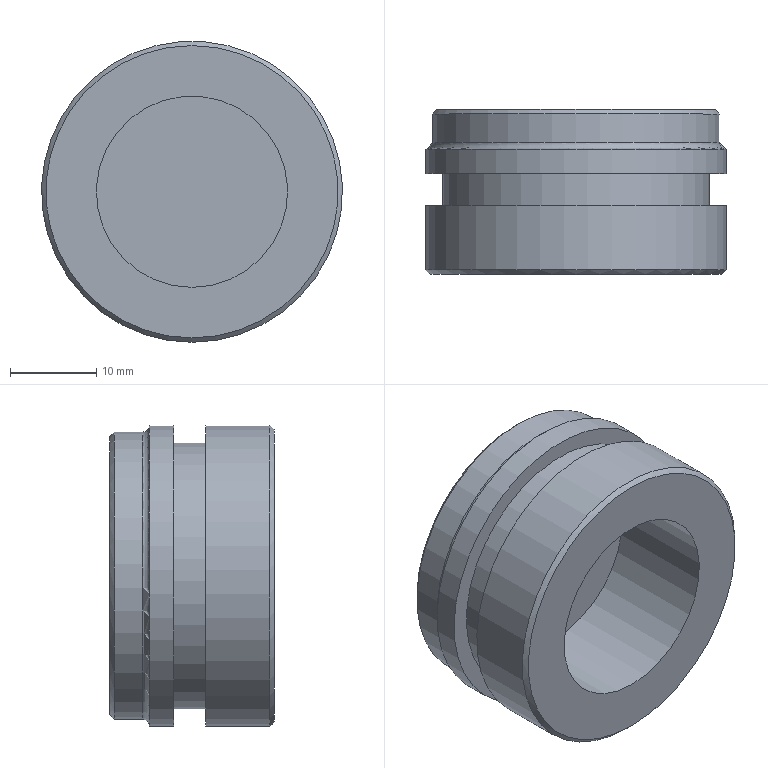Part | NX | features MG0330 trunion parts 24(stanchion group) 2 | 1 solid | 13 faces | box 34.849 x 19.05 x 34.849 mm | volume 12105 mm3 | cylinder 5 | plane 5 | cone 2 | torus 1 | commonest cylinder face diameters 34.849 x2 22.149 x1 30.836 x1 33.261 x1
STEP:
#1=CARTESIAN_POINT('',(0.,267.208,-17.424));
#2=VERTEX_POINT('',#1);
#3=CARTESIAN_POINT('',(0.,267.208,0.));
#4=DIRECTION('',(0.,-1.,0.));
#5=DIRECTION('',(0.,0.,-1.));
#6=AXIS2_PLACEMENT_3D('',#3,#4,#5);
#7=CIRCLE('',#6,17.424);
#8=EDGE_CURVE('',#2,#2,#7,.F.);
#9=ORIENTED_EDGE('',*,*,#8,.T.);
#10=EDGE_LOOP('',(#9));
#11=FACE_BOUND('',#10,.T.);
#12=CARTESIAN_POINT('',(0.,274.65,-17.424));
#13=VERTEX_POINT('',#12);
#14=CARTESIAN_POINT('',(0.,274.65,0.));
#15=DIRECTION('',(0.,-1.,0.));
#16=DIRECTION('',(0.,0.,-1.));
#17=AXIS2_PLACEMENT_3D('',#14,#15,#16);
#18=CIRCLE('',#17,17.424);
#19=EDGE_CURVE('',#13,#13,#18,.T.);
#20=ORIENTED_EDGE('',*,*,#19,.T.);
#21=EDGE_LOOP('',(#20));
#22=FACE_BOUND('',#21,.T.);
#23=CARTESIAN_POINT('',(0.,276.225,0.));
#24=DIRECTION('',(0.,-1.,0.));
#25=DIRECTION('',(0.,0.,-1.));
#26=AXIS2_PLACEMENT_3D('',#23,#24,#25);
#27=CYLINDRICAL_SURFACE('',#26,17.424);
#28=ADVANCED_FACE('',(#11,#22),#27,.T.);
#29=CARTESIAN_POINT('',(0.,274.65,-15.418));
#30=VERTEX_POINT('',#29);
#31=CARTESIAN_POINT('',(0.,274.65,0.));
#32=DIRECTION('',(0.,-1.,0.));
#33=DIRECTION('',(0.,0.,-1.));
#34=AXIS2_PLACEMENT_3D('',#31,#32,#33);
#35=CIRCLE('',#34,15.418);
#36=EDGE_CURVE('',#30,#30,#35,.T.);
#37=ORIENTED_EDGE('',*,*,#36,.T.);
#38=EDGE_LOOP('',(#37));
#39=FACE_BOUND('',#38,.T.);
#40=ORIENTED_EDGE('',*,*,#19,.F.);
#41=EDGE_LOOP('',(#40));
#42=FACE_BOUND('',#41,.T.);
#43=CARTESIAN_POINT('',(17.424,274.65,0.));
#44=DIRECTION('',(0.,1.,0.));
#45=DIRECTION('',(0.,0.,1.));
#46=AXIS2_PLACEMENT_3D('',#43,#44,#45);
#47=PLANE('',#46);
#48=ADVANCED_FACE('',(#39,#42),#47,.T.);
#49=CARTESIAN_POINT('',(0.,278.359,-15.418));
#50=VERTEX_POINT('',#49);
#51=CARTESIAN_POINT('',(0.,278.359,0.));
#52=DIRECTION('',(0.,-1.,0.));
#53=DIRECTION('',(0.,0.,-1.));
#54=AXIS2_PLACEMENT_3D('',#51,#52,#53);
#55=CIRCLE('',#54,15.418);
#56=EDGE_CURVE('',#50,#50,#55,.T.);
#57=ORIENTED_EDGE('',*,*,#56,.T.);
#58=EDGE_LOOP('',(#57));
#59=FACE_BOUND('',#58,.T.);
#60=ORIENTED_EDGE('',*,*,#36,.F.);
#61=EDGE_LOOP('',(#60));
#62=FACE_BOUND('',#61,.T.);
#63=CARTESIAN_POINT('',(0.,276.225,0.));
#64=DIRECTION('',(0.,-1.,0.));
#65=DIRECTION('',(0.,0.,-1.));
#66=AXIS2_PLACEMENT_3D('',#63,#64,#65);
#67=CYLINDRICAL_SURFACE('',#66,15.418);
#68=ADVANCED_FACE('',(#59,#62),#67,.T.);
#69=CARTESIAN_POINT('',(0.,278.359,-17.424));
#70=VERTEX_POINT('',#69);
#71=CARTESIAN_POINT('',(0.,278.359,0.));
#72=DIRECTION('',(0.,-1.,0.));
#73=DIRECTION('',(0.,0.,-1.));
#74=AXIS2_PLACEMENT_3D('',#71,#72,#73);
#75=CIRCLE('',#74,17.424);
#76=EDGE_CURVE('',#70,#70,#75,.T.);
#77=ORIENTED_EDGE('',*,*,#76,.T.);
#78=EDGE_LOOP('',(#77));
#79=FACE_BOUND('',#78,.T.);
#80=ORIENTED_EDGE('',*,*,#56,.F.);
#81=EDGE_LOOP('',(#80));
#82=FACE_BOUND('',#81,.T.);
#83=CARTESIAN_POINT('',(17.424,278.359,0.));
#84=DIRECTION('',(0.,-1.,0.));
#85=DIRECTION('',(0.,0.,-1.));
#86=AXIS2_PLACEMENT_3D('',#83,#84,#85);
#87=PLANE('',#86);
#88=ADVANCED_FACE('',(#79,#82),#87,.T.);
#89=CARTESIAN_POINT('',(0.,281.146,-17.424));
#90=VERTEX_POINT('',#89);
#91=CARTESIAN_POINT('',(0.,281.146,0.));
#92=DIRECTION('',(0.,-1.,0.));
#93=DIRECTION('',(0.,0.,-1.));
#94=AXIS2_PLACEMENT_3D('',#91,#92,#93);
#95=CIRCLE('',#94,17.424);
#96=EDGE_CURVE('',#90,#90,#95,.T.);
#97=ORIENTED_EDGE('',*,*,#96,.T.);
#98=EDGE_LOOP('',(#97));
#99=FACE_BOUND('',#98,.T.);
#100=ORIENTED_EDGE('',*,*,#76,.F.);
#101=EDGE_LOOP('',(#100));
#102=FACE_BOUND('',#101,.T.);
#103=CARTESIAN_POINT('',(0.,276.225,0.));
#104=DIRECTION('',(0.,-1.,0.));
#105=DIRECTION('',(0.,0.,-1.));
#106=AXIS2_PLACEMENT_3D('',#103,#104,#105);
#107=CYLINDRICAL_SURFACE('',#106,17.424);
#108=ADVANCED_FACE('',(#99,#102),#107,.T.);
#109=CARTESIAN_POINT('',(0.,281.94,-16.631));
#110=VERTEX_POINT('',#109);
#111=CARTESIAN_POINT('',(0.,281.94,0.));
#112=DIRECTION('',(0.,-1.,0.));
#113=DIRECTION('',(0.,0.,-1.));
#114=AXIS2_PLACEMENT_3D('',#111,#112,#113);
#115=CIRCLE('',#114,16.631);
#116=EDGE_CURVE('',#110,#110,#115,.T.);
#117=ORIENTED_EDGE('',*,*,#116,.T.);
#118=EDGE_LOOP('',(#117));
#119=FACE_BOUND('',#118,.T.);
#120=ORIENTED_EDGE('',*,*,#96,.F.);
#121=EDGE_LOOP('',(#120));
#122=FACE_BOUND('',#121,.T.);
#123=CARTESIAN_POINT('',(0.,281.94,0.));
#124=DIRECTION('',(0.,-1.,0.));
#125=DIRECTION('',(0.,0.,-1.));
#126=AXIS2_PLACEMENT_3D('',#123,#124,#125);
#127=TOROIDAL_SURFACE('',#126,17.424,0.7937);
#128=ADVANCED_FACE('',(#119,#122),#127,.F.);
#129=CARTESIAN_POINT('',(0.,285.242,16.631));
#130=VERTEX_POINT('',#129);
#131=CARTESIAN_POINT('',(0.,285.242,0.));
#132=DIRECTION('',(0.,1.,0.));
#133=DIRECTION('',(0.,0.,1.));
#134=AXIS2_PLACEMENT_3D('',#131,#132,#133);
#135=CIRCLE('',#134,16.631);
#136=EDGE_CURVE('',#130,#130,#135,.F.);
#137=ORIENTED_EDGE('',*,*,#136,.T.);
#138=EDGE_LOOP('',(#137));
#139=FACE_BOUND('',#138,.T.);
#140=ORIENTED_EDGE('',*,*,#116,.F.);
#141=EDGE_LOOP('',(#140));
#142=FACE_BOUND('',#141,.T.);
#143=CARTESIAN_POINT('',(0.,276.225,0.));
#144=DIRECTION('',(0.,-1.,0.));
#145=DIRECTION('',(0.,0.,-1.));
#146=AXIS2_PLACEMENT_3D('',#143,#144,#145);
#147=CYLINDRICAL_SURFACE('',#146,16.631);
#148=ADVANCED_FACE('',(#139,#142),#147,.T.);
#149=CARTESIAN_POINT('',(0.,285.75,16.123));
#150=VERTEX_POINT('',#149);
#151=CARTESIAN_POINT('',(0.,285.75,0.));
#152=DIRECTION('',(0.,1.,0.));
#153=DIRECTION('',(0.,0.,1.));
#154=AXIS2_PLACEMENT_3D('',#151,#152,#153);
#155=CIRCLE('',#154,16.123);
#156=EDGE_CURVE('',#150,#150,#155,.T.);
#157=ORIENTED_EDGE('',*,*,#156,.T.);
#158=EDGE_LOOP('',(#157));
#159=FACE_BOUND('',#158,.T.);
#160=CARTESIAN_POINT('',(16.631,285.75,0.));
#161=DIRECTION('',(0.,1.,0.));
#162=DIRECTION('',(0.,0.,1.));
#163=AXIS2_PLACEMENT_3D('',#160,#161,#162);
#164=PLANE('',#163);
#165=ADVANCED_FACE('',(#159),#164,.T.);
#166=CARTESIAN_POINT('',(0.,279.4,-11.074));
#167=VERTEX_POINT('',#166);
#168=CARTESIAN_POINT('',(0.,279.4,0.));
#169=DIRECTION('',(0.,-1.,0.));
#170=DIRECTION('',(0.,0.,-1.));
#171=AXIS2_PLACEMENT_3D('',#168,#169,#170);
#172=CIRCLE('',#171,11.074);
#173=EDGE_CURVE('',#167,#167,#172,.T.);
#174=ORIENTED_EDGE('',*,*,#173,.T.);
#175=EDGE_LOOP('',(#174));
#176=FACE_BOUND('',#175,.T.);
#177=CARTESIAN_POINT('',(11.074,279.4,0.));
#178=DIRECTION('',(0.,-1.,0.));
#179=DIRECTION('',(0.,0.,-1.));
#180=AXIS2_PLACEMENT_3D('',#177,#178,#179);
#181=PLANE('',#180);
#182=ADVANCED_FACE('',(#176),#181,.T.);
#183=CARTESIAN_POINT('',(0.,266.7,-11.074));
#184=VERTEX_POINT('',#183);
#185=CARTESIAN_POINT('',(0.,266.7,0.));
#186=DIRECTION('',(0.,-1.,0.));
#187=DIRECTION('',(0.,0.,-1.));
#188=AXIS2_PLACEMENT_3D('',#185,#186,#187);
#189=CIRCLE('',#188,11.074);
#190=EDGE_CURVE('',#184,#184,#189,.T.);
#191=ORIENTED_EDGE('',*,*,#190,.T.);
#192=EDGE_LOOP('',(#191));
#193=FACE_BOUND('',#192,.T.);
#194=ORIENTED_EDGE('',*,*,#173,.F.);
#195=EDGE_LOOP('',(#194));
#196=FACE_BOUND('',#195,.T.);
#197=CARTESIAN_POINT('',(0.,276.225,0.));
#198=DIRECTION('',(0.,-1.,0.));
#199=DIRECTION('',(0.,0.,-1.));
#200=AXIS2_PLACEMENT_3D('',#197,#198,#199);
#201=CYLINDRICAL_SURFACE('',#200,11.074);
#202=ADVANCED_FACE('',(#193,#196),#201,.F.);
#203=CARTESIAN_POINT('',(0.,266.7,-16.916));
#204=VERTEX_POINT('',#203);
#205=CARTESIAN_POINT('',(0.,266.7,0.));
#206=DIRECTION('',(0.,-1.,0.));
#207=DIRECTION('',(0.,0.,-1.));
#208=AXIS2_PLACEMENT_3D('',#205,#206,#207);
#209=CIRCLE('',#208,16.916);
#210=EDGE_CURVE('',#204,#204,#209,.T.);
#211=ORIENTED_EDGE('',*,*,#210,.T.);
#212=EDGE_LOOP('',(#211));
#213=FACE_BOUND('',#212,.T.);
#214=ORIENTED_EDGE('',*,*,#190,.F.);
#215=EDGE_LOOP('',(#214));
#216=FACE_BOUND('',#215,.T.);
#217=CARTESIAN_POINT('',(11.074,266.7,0.));
#218=DIRECTION('',(0.,-1.,0.));
#219=DIRECTION('',(0.,0.,-1.));
#220=AXIS2_PLACEMENT_3D('',#217,#218,#219);
#221=PLANE('',#220);
#222=ADVANCED_FACE('',(#213,#216),#221,.T.);
#223=ORIENTED_EDGE('',*,*,#156,.F.);
#224=EDGE_LOOP('',(#223));
#225=FACE_BOUND('',#224,.T.);
#226=ORIENTED_EDGE('',*,*,#136,.F.);
#227=EDGE_LOOP('',(#226));
#228=FACE_BOUND('',#227,.T.);
#229=CARTESIAN_POINT('',(0.,285.242,0.));
#230=DIRECTION('',(0.,-1.,0.));
#231=DIRECTION('',(0.,0.,-1.));
#232=AXIS2_PLACEMENT_3D('',#229,#230,#231);
#233=CONICAL_SURFACE('',#232,16.631,0.7854);
#234=ADVANCED_FACE('',(#225,#228),#233,.T.);
#235=ORIENTED_EDGE('',*,*,#8,.F.);
#236=EDGE_LOOP('',(#235));
#237=FACE_BOUND('',#236,.T.);
#238=ORIENTED_EDGE('',*,*,#210,.F.);
#239=EDGE_LOOP('',(#238));
#240=FACE_BOUND('',#239,.T.);
#241=CARTESIAN_POINT('',(0.,266.7,0.));
#242=DIRECTION('',(0.,1.,0.));
#243=DIRECTION('',(0.,0.,1.));
#244=AXIS2_PLACEMENT_3D('',#241,#242,#243);
#245=CONICAL_SURFACE('',#244,16.916,0.7854);
#246=ADVANCED_FACE('',(#237,#240),#245,.T.);
#247=CLOSED_SHELL('',(#28,#48,#68,#88,#108,#128,#148,#165,#182,#202,#222,#234,#246));
#248=MANIFOLD_SOLID_BREP('',#247);
#249=(LENGTH_UNIT()NAMED_UNIT(*)SI_UNIT(.MILLI.,.METRE.));
#250=UNCERTAINTY_MEASURE_WITH_UNIT(LENGTH_MEASURE(0.00001),#249,'','');
#251=(NAMED_UNIT(*)PLANE_ANGLE_UNIT()SI_UNIT($,.RADIAN.));
#252=(NAMED_UNIT(*)SI_UNIT($,.STERADIAN.)SOLID_ANGLE_UNIT());
#253=(GEOMETRIC_REPRESENTATION_CONTEXT(3)GLOBAL_UNCERTAINTY_ASSIGNED_CONTEXT((#250))GLOBAL_UNIT_ASSIGNED_CONTEXT((#249,#251,#252))REPRESENTATION_CONTEXT('',''));
#254=ADVANCED_BREP_SHAPE_REPRESENTATION('',(#248),#253);